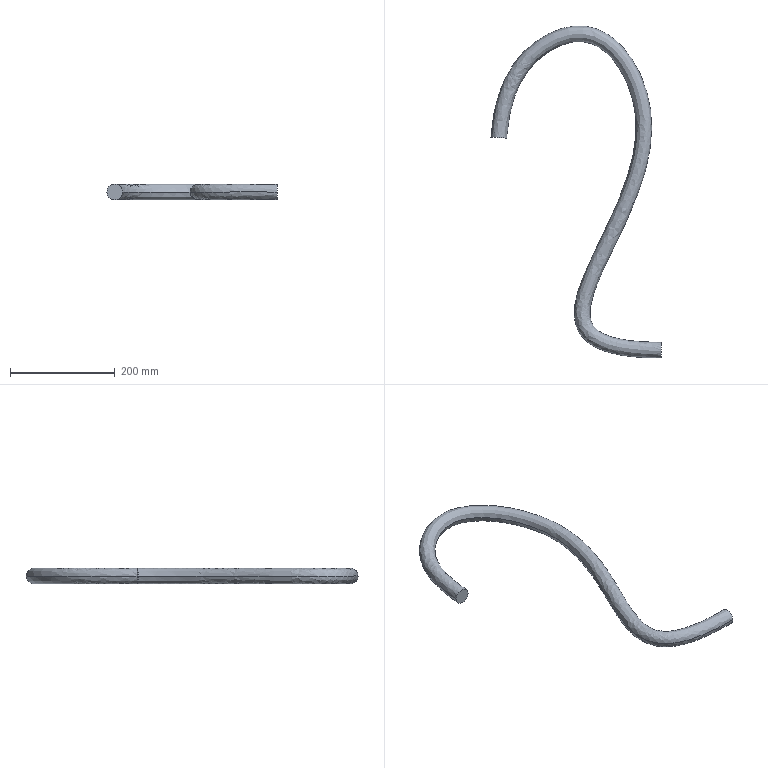Part | STEP file | 1 solid | 4 faces | box 324.826 x 634.125 x 30 mm | volume 760478 mm3 | spline 2 | plane 2